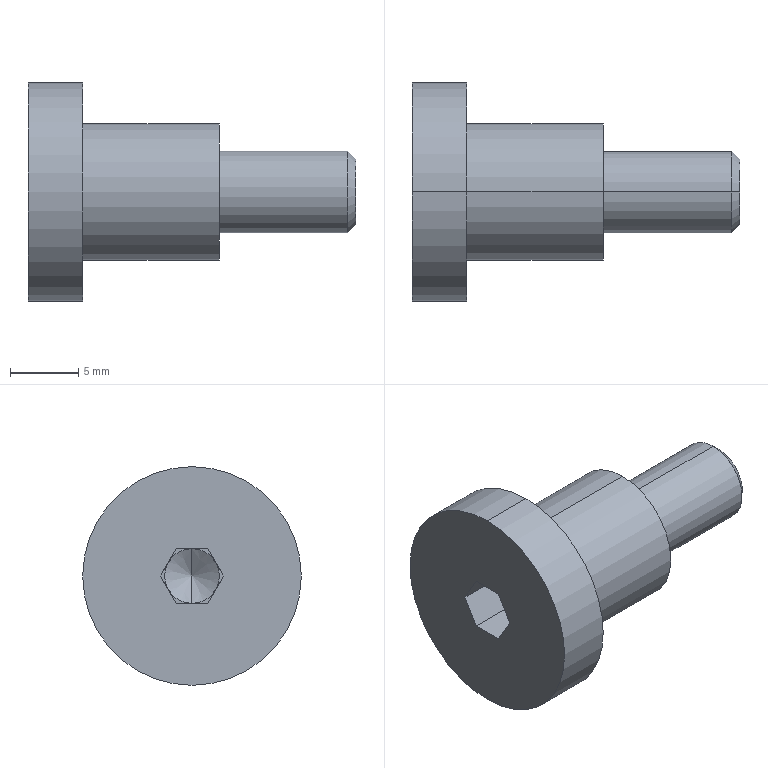Part | STEP file | 0217_003_DBTS6-10-10 | 1 solid | 26 faces | box 24 x 16 x 16 mm | volume 1816 mm3 | plane 16 | cylinder 6 | cone 4 | commonest cylinder face diameters 6 x2 10 x2 16 x2